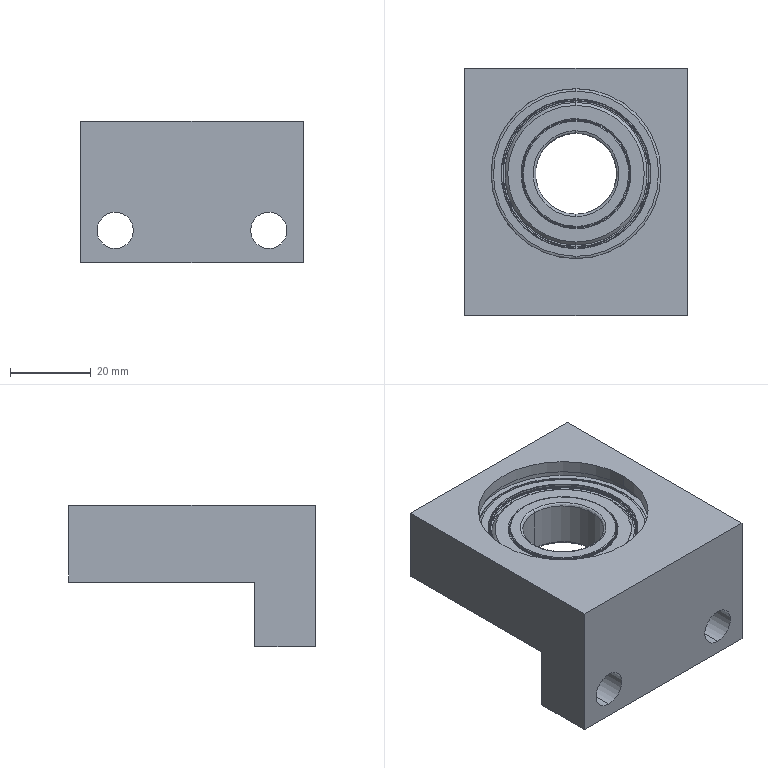Part | SolidWorks | features BaseBody 2 | 2 solids | 159 faces | box 55 x 61 x 35 mm | volume 59445 mm3 | spline 52 | cylinder 44 | cone 40 | plane 23 | commonest cylinder face diameters 42 x6 9 x4 25.6 x4 26.4 x4 26.8 x4 27.2 x4